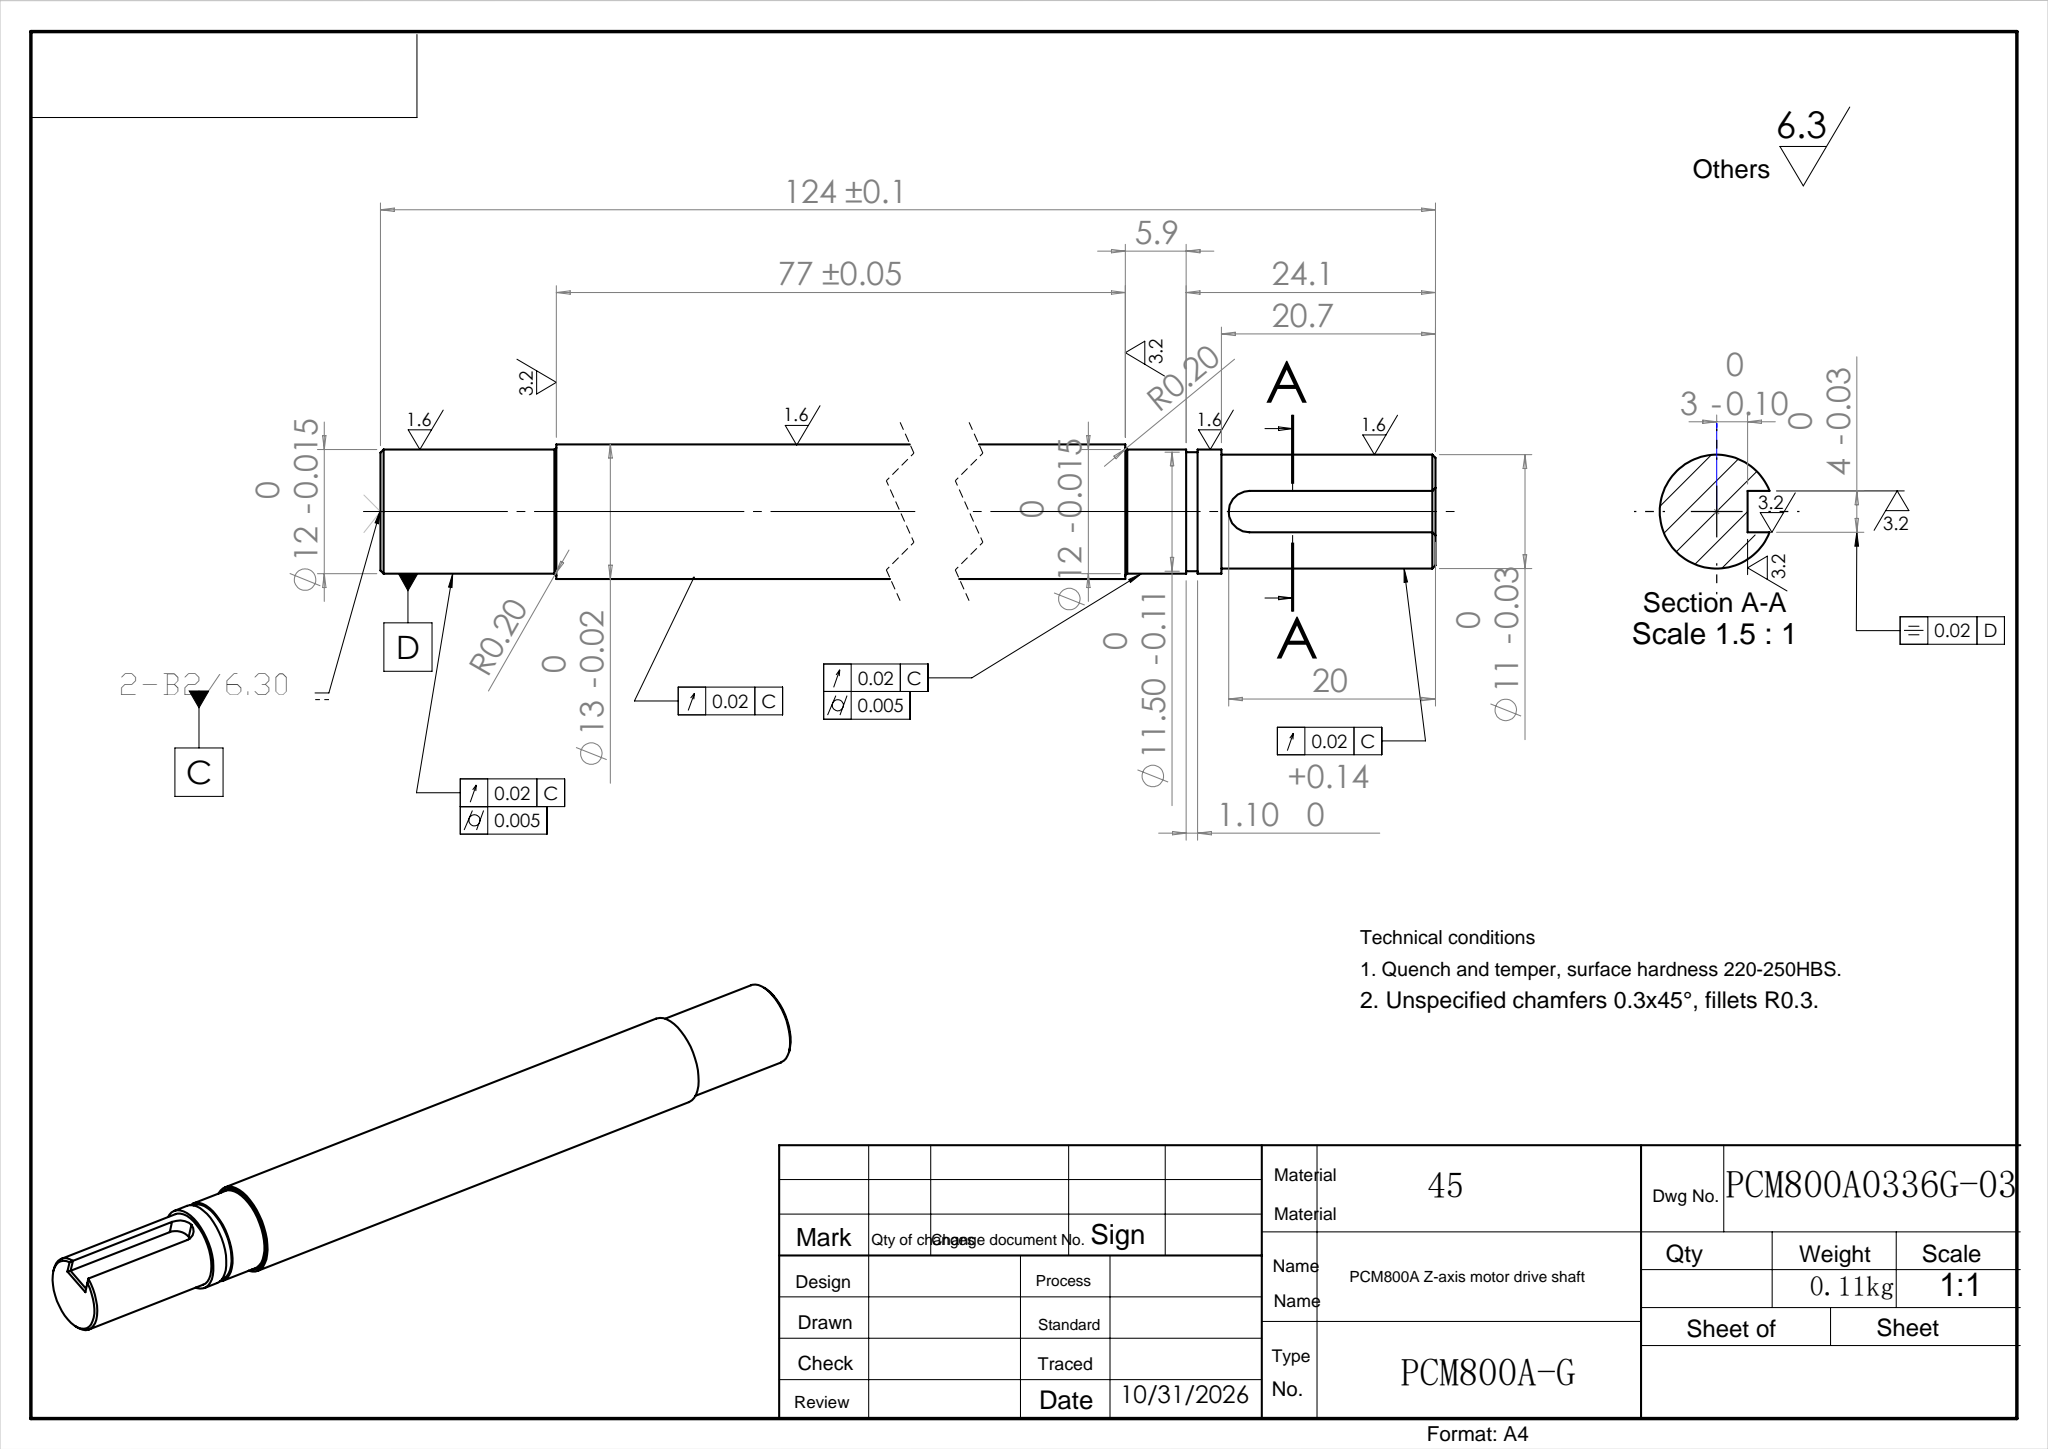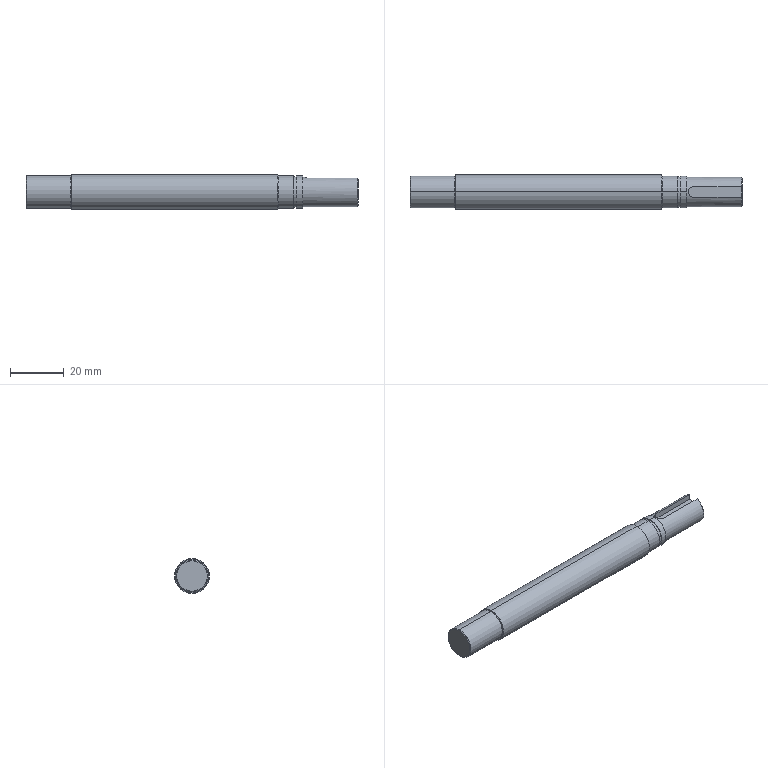Part | SolidWorks | features Boss 6, Fillet 3, Chamfer 1, Cut 1 | 1 solid | 34 faces | box 124 x 13 x 13 mm | volume 14963 mm3 | cylinder 14 | plane 13 | torus 4 | cone 3 | commonest cylinder face diameters 12 x6 4 x2 11 x2 11.5 x2 13 x2
STEP:
#1=CARTESIAN_POINT('',(77.2,0.,6.));
#2=VERTEX_POINT('',#1);
#3=CARTESIAN_POINT('',(77.2,0.,-6.));
#4=VERTEX_POINT('',#3);
#5=CARTESIAN_POINT('',(77.2,0.,0.));
#6=DIRECTION('',(1.,0.,0.));
#7=DIRECTION('',(0.,0.,-1.));
#8=AXIS2_PLACEMENT_3D('',#5,#6,#7);
#9=CIRCLE('',#8,6.);
#10=EDGE_CURVE('',#2,#4,#9,.T.);
#11=ORIENTED_EDGE('',*,*,#10,.F.);
#12=CARTESIAN_POINT('',(77.,0.,6.2));
#13=VERTEX_POINT('',#12);
#14=CARTESIAN_POINT('',(77.2,0.,6.2));
#15=DIRECTION('',(0.,1.,0.));
#16=DIRECTION('',(0.,0.,1.));
#17=AXIS2_PLACEMENT_3D('',#14,#15,#16);
#18=CIRCLE('',#17,0.2);
#19=EDGE_CURVE('',#2,#13,#18,.T.);
#20=ORIENTED_EDGE('',*,*,#19,.T.);
#21=CARTESIAN_POINT('',(77.,0.,-6.2));
#22=VERTEX_POINT('',#21);
#23=CARTESIAN_POINT('',(77.,0.,0.));
#24=DIRECTION('',(-1.,0.,0.));
#25=DIRECTION('',(0.,0.,-1.));
#26=AXIS2_PLACEMENT_3D('',#23,#24,#25);
#27=CIRCLE('',#26,6.2);
#28=EDGE_CURVE('',#22,#13,#27,.T.);
#29=ORIENTED_EDGE('',*,*,#28,.F.);
#30=CARTESIAN_POINT('',(77.2,0.,-6.2));
#31=DIRECTION('',(0.,-1.,0.));
#32=DIRECTION('',(0.,0.,-1.));
#33=AXIS2_PLACEMENT_3D('',#30,#31,#32);
#34=CIRCLE('',#33,0.2);
#35=EDGE_CURVE('',#4,#22,#34,.T.);
#36=ORIENTED_EDGE('',*,*,#35,.F.);
#37=EDGE_LOOP('',(#11,#20,#29,#36));
#38=FACE_OUTER_BOUND('',#37,.T.);
#39=CARTESIAN_POINT('',(77.2,0.,0.));
#40=DIRECTION('',(1.,0.,0.));
#41=DIRECTION('',(0.,0.,-1.));
#42=AXIS2_PLACEMENT_3D('',#39,#40,#41);
#43=TOROIDAL_SURFACE('',#42,6.2,0.2);
#44=ADVANCED_FACE('',(#38),#43,.F.);
#45=CARTESIAN_POINT('',(0.,0.,6.2));
#46=VERTEX_POINT('',#45);
#47=CARTESIAN_POINT('',(0.,0.,-6.2));
#48=VERTEX_POINT('',#47);
#49=CARTESIAN_POINT('',(0.,0.,0.));
#50=DIRECTION('',(1.,0.,0.));
#51=DIRECTION('',(0.,0.,-1.));
#52=AXIS2_PLACEMENT_3D('',#49,#50,#51);
#53=CIRCLE('',#52,6.2);
#54=EDGE_CURVE('',#46,#48,#53,.T.);
#55=ORIENTED_EDGE('',*,*,#54,.F.);
#56=CARTESIAN_POINT('',(-0.2,0.,6.));
#57=VERTEX_POINT('',#56);
#58=CARTESIAN_POINT('',(-0.2,0.,6.2));
#59=DIRECTION('',(0.,1.,0.));
#60=DIRECTION('',(0.,0.,1.));
#61=AXIS2_PLACEMENT_3D('',#58,#59,#60);
#62=CIRCLE('',#61,0.2);
#63=EDGE_CURVE('',#46,#57,#62,.T.);
#64=ORIENTED_EDGE('',*,*,#63,.T.);
#65=CARTESIAN_POINT('',(-0.2,0.,-6.));
#66=VERTEX_POINT('',#65);
#67=CARTESIAN_POINT('',(-0.2,0.,0.));
#68=DIRECTION('',(-1.,0.,0.));
#69=DIRECTION('',(0.,0.,-1.));
#70=AXIS2_PLACEMENT_3D('',#67,#68,#69);
#71=CIRCLE('',#70,6.);
#72=EDGE_CURVE('',#66,#57,#71,.T.);
#73=ORIENTED_EDGE('',*,*,#72,.F.);
#74=CARTESIAN_POINT('',(-0.2,0.,-6.2));
#75=DIRECTION('',(0.,-1.,0.));
#76=DIRECTION('',(0.,0.,-1.));
#77=AXIS2_PLACEMENT_3D('',#74,#75,#76);
#78=CIRCLE('',#77,0.2);
#79=EDGE_CURVE('',#48,#66,#78,.T.);
#80=ORIENTED_EDGE('',*,*,#79,.F.);
#81=EDGE_LOOP('',(#55,#64,#73,#80));
#82=FACE_OUTER_BOUND('',#81,.T.);
#83=CARTESIAN_POINT('',(-0.2,0.,0.));
#84=DIRECTION('',(1.,0.,0.));
#85=DIRECTION('',(0.,0.,-1.));
#86=AXIS2_PLACEMENT_3D('',#83,#84,#85);
#87=TOROIDAL_SURFACE('',#86,6.2,0.2);
#88=ADVANCED_FACE('',(#82),#87,.F.);
#89=CARTESIAN_POINT('',(-17.,0.,5.7));
#90=VERTEX_POINT('',#89);
#91=CARTESIAN_POINT('',(-17.,0.,-5.7));
#92=VERTEX_POINT('',#91);
#93=CARTESIAN_POINT('',(-17.,0.,0.));
#94=DIRECTION('',(-1.,0.,0.));
#95=DIRECTION('',(0.,0.,1.));
#96=AXIS2_PLACEMENT_3D('',#93,#94,#95);
#97=CIRCLE('',#96,5.7);
#98=EDGE_CURVE('',#90,#92,#97,.T.);
#99=ORIENTED_EDGE('',*,*,#98,.F.);
#100=CARTESIAN_POINT('',(-16.7,0.,6.));
#101=VERTEX_POINT('',#100);
#102=CARTESIAN_POINT('',(-17.,0.,5.7));
#103=DIRECTION('',(0.7071,0.,0.7071));
#104=VECTOR('',#103,1000.);
#105=LINE('',#102,#104);
#106=EDGE_CURVE('',#90,#101,#105,.T.);
#107=ORIENTED_EDGE('',*,*,#106,.T.);
#108=CARTESIAN_POINT('',(-16.7,0.,-6.));
#109=VERTEX_POINT('',#108);
#110=CARTESIAN_POINT('',(-16.7,0.,0.));
#111=DIRECTION('',(1.,0.,0.));
#112=DIRECTION('',(0.,0.,1.));
#113=AXIS2_PLACEMENT_3D('',#110,#111,#112);
#114=CIRCLE('',#113,6.);
#115=EDGE_CURVE('',#109,#101,#114,.T.);
#116=ORIENTED_EDGE('',*,*,#115,.F.);
#117=CARTESIAN_POINT('',(-17.,0.,-5.7));
#118=DIRECTION('',(0.7071,0.,-0.7071));
#119=VECTOR('',#118,1000.);
#120=LINE('',#117,#119);
#121=EDGE_CURVE('',#92,#109,#120,.T.);
#122=ORIENTED_EDGE('',*,*,#121,.F.);
#123=EDGE_LOOP('',(#99,#107,#116,#122));
#124=FACE_OUTER_BOUND('',#123,.T.);
#125=CARTESIAN_POINT('',(-17.,0.,0.));
#126=DIRECTION('',(1.,0.,0.));
#127=DIRECTION('',(0.,0.,-1.));
#128=AXIS2_PLACEMENT_3D('',#125,#126,#127);
#129=CONICAL_SURFACE('',#128,5.7,0.7854);
#130=ADVANCED_FACE('',(#124),#129,.T.);
#131=ORIENTED_EDGE('',*,*,#115,.T.);
#132=CARTESIAN_POINT('',(-17.,0.,6.));
#133=DIRECTION('',(1.,0.,0.));
#134=VECTOR('',#133,1000.);
#135=LINE('',#132,#134);
#136=EDGE_CURVE('',#101,#57,#135,.T.);
#137=ORIENTED_EDGE('',*,*,#136,.T.);
#138=CARTESIAN_POINT('',(-0.2,0.,0.));
#139=DIRECTION('',(-1.,0.,0.));
#140=DIRECTION('',(0.,0.,-1.));
#141=AXIS2_PLACEMENT_3D('',#138,#139,#140);
#142=CIRCLE('',#141,6.);
#143=EDGE_CURVE('',#57,#66,#142,.T.);
#144=ORIENTED_EDGE('',*,*,#143,.T.);
#145=CARTESIAN_POINT('',(-17.,0.,-6.));
#146=DIRECTION('',(1.,0.,0.));
#147=VECTOR('',#146,1000.);
#148=LINE('',#145,#147);
#149=EDGE_CURVE('',#109,#66,#148,.T.);
#150=ORIENTED_EDGE('',*,*,#149,.F.);
#151=EDGE_LOOP('',(#131,#137,#144,#150));
#152=FACE_OUTER_BOUND('',#151,.T.);
#153=CARTESIAN_POINT('',(-17.,0.,0.));
#154=DIRECTION('',(1.,0.,0.));
#155=DIRECTION('',(0.,0.,-1.));
#156=AXIS2_PLACEMENT_3D('',#153,#154,#155);
#157=CYLINDRICAL_SURFACE('',#156,6.);
#158=ADVANCED_FACE('',(#152),#157,.T.);
#159=CARTESIAN_POINT('',(106.7,2.,5.123));
#160=VERTEX_POINT('',#159);
#161=CARTESIAN_POINT('',(106.7,0.,-5.5));
#162=VERTEX_POINT('',#161);
#163=CARTESIAN_POINT('',(106.7,0.,0.));
#164=DIRECTION('',(-1.,0.,0.));
#165=DIRECTION('',(0.,0.,-1.));
#166=AXIS2_PLACEMENT_3D('',#163,#164,#165);
#167=CIRCLE('',#166,5.5);
#168=EDGE_CURVE('',#160,#162,#167,.T.);
#169=ORIENTED_EDGE('',*,*,#168,.T.);
#170=CARTESIAN_POINT('',(86.3,0.,-5.5));
#171=VERTEX_POINT('',#170);
#172=CARTESIAN_POINT('',(107.,0.,-5.5));
#173=DIRECTION('',(-1.,0.,0.));
#174=VECTOR('',#173,1000.);
#175=LINE('',#172,#174);
#176=EDGE_CURVE('',#162,#171,#175,.T.);
#177=ORIENTED_EDGE('',*,*,#176,.T.);
#178=CARTESIAN_POINT('',(86.3,0.,5.5));
#179=VERTEX_POINT('',#178);
#180=CARTESIAN_POINT('',(86.3,0.,0.));
#181=DIRECTION('',(1.,0.,0.));
#182=DIRECTION('',(0.,0.,-1.));
#183=AXIS2_PLACEMENT_3D('',#180,#181,#182);
#184=CIRCLE('',#183,5.5);
#185=EDGE_CURVE('',#171,#179,#184,.T.);
#186=ORIENTED_EDGE('',*,*,#185,.T.);
#187=CARTESIAN_POINT('',(87.,0.,5.5));
#188=VERTEX_POINT('',#187);
#189=CARTESIAN_POINT('',(107.,0.,5.5));
#190=DIRECTION('',(-1.,0.,0.));
#191=VECTOR('',#190,1000.);
#192=LINE('',#189,#191);
#193=EDGE_CURVE('',#188,#179,#192,.T.);
#194=ORIENTED_EDGE('',*,*,#193,.F.);
#195=CARTESIAN_POINT('',(89.,2.,5.123));
#196=VERTEX_POINT('',#195);
#197=CARTESIAN_POINT('',(87.,0.,5.5));
#198=CARTESIAN_POINT('',(87.,0.1333,5.5));
#199=CARTESIAN_POINT('',(87.013,0.2641,5.495));
#200=CARTESIAN_POINT('',(87.065,0.5212,5.477));
#201=CARTESIAN_POINT('',(87.104,0.6488,5.463));
#202=CARTESIAN_POINT('',(87.204,0.8905,5.429));
#203=CARTESIAN_POINT('',(87.266,1.005,5.409));
#204=CARTESIAN_POINT('',(87.411,1.221,5.364));
#205=CARTESIAN_POINT('',(87.494,1.323,5.339));
#206=CARTESIAN_POINT('',(87.769,1.597,5.266));
#207=CARTESIAN_POINT('',(87.989,1.745,5.217));
#208=CARTESIAN_POINT('',(88.349,1.896,5.163));
#209=CARTESIAN_POINT('',(88.476,1.935,5.149));
#210=CARTESIAN_POINT('',(88.735,1.987,5.129));
#211=CARTESIAN_POINT('',(88.867,2.,5.123));
#212=CARTESIAN_POINT('',(89.,2.,5.123));
#213=B_SPLINE_CURVE_WITH_KNOTS('',3,(#197,#198,#199,#200,#201,#202,#203,#204,#205,#206,#207,#208,#209,#210,#211,#212),.UNSPECIFIED.,.F.,.F.,(4,2,2,2,2,2,2,4),(0.,0.000394,0.0007879,0.001182,0.001576,0.002364,0.002758,0.003152),.UNSPECIFIED.);
#214=EDGE_CURVE('',#188,#196,#213,.T.);
#215=ORIENTED_EDGE('',*,*,#214,.T.);
#216=CARTESIAN_POINT('',(87.,2.,5.123));
#217=DIRECTION('',(1.,0.,0.));
#218=VECTOR('',#217,1000.);
#219=LINE('',#216,#218);
#220=EDGE_CURVE('',#196,#160,#219,.T.);
#221=ORIENTED_EDGE('',*,*,#220,.T.);
#222=EDGE_LOOP('',(#169,#177,#186,#194,#215,#221));
#223=FACE_OUTER_BOUND('',#222,.T.);
#224=CARTESIAN_POINT('',(107.,0.,0.));
#225=DIRECTION('',(-1.,0.,0.));
#226=DIRECTION('',(0.,0.,1.));
#227=AXIS2_PLACEMENT_3D('',#224,#225,#226);
#228=CYLINDRICAL_SURFACE('',#227,5.5);
#229=ADVANCED_FACE('',(#223),#228,.T.);
#230=CARTESIAN_POINT('',(86.3,0.,-6.));
#231=VERTEX_POINT('',#230);
#232=CARTESIAN_POINT('',(86.3,0.,6.));
#233=VERTEX_POINT('',#232);
#234=CARTESIAN_POINT('',(86.3,0.,0.));
#235=DIRECTION('',(1.,0.,0.));
#236=DIRECTION('',(0.,0.,-1.));
#237=AXIS2_PLACEMENT_3D('',#234,#235,#236);
#238=CIRCLE('',#237,6.);
#239=EDGE_CURVE('',#231,#233,#238,.T.);
#240=ORIENTED_EDGE('',*,*,#239,.F.);
#241=CARTESIAN_POINT('',(84.,0.,-6.));
#242=VERTEX_POINT('',#241);
#243=CARTESIAN_POINT('',(86.3,0.,-6.));
#244=DIRECTION('',(-1.,0.,0.));
#245=VECTOR('',#244,1000.);
#246=LINE('',#243,#245);
#247=EDGE_CURVE('',#231,#242,#246,.T.);
#248=ORIENTED_EDGE('',*,*,#247,.T.);
#249=CARTESIAN_POINT('',(84.,0.,6.));
#250=VERTEX_POINT('',#249);
#251=CARTESIAN_POINT('',(84.,0.,0.));
#252=DIRECTION('',(1.,0.,0.));
#253=DIRECTION('',(0.,0.,-1.));
#254=AXIS2_PLACEMENT_3D('',#251,#252,#253);
#255=CIRCLE('',#254,6.);
#256=EDGE_CURVE('',#242,#250,#255,.T.);
#257=ORIENTED_EDGE('',*,*,#256,.T.);
#258=CARTESIAN_POINT('',(86.3,0.,6.));
#259=DIRECTION('',(-1.,0.,0.));
#260=VECTOR('',#259,1000.);
#261=LINE('',#258,#260);
#262=EDGE_CURVE('',#233,#250,#261,.T.);
#263=ORIENTED_EDGE('',*,*,#262,.F.);
#264=EDGE_LOOP('',(#240,#248,#257,#263));
#265=FACE_OUTER_BOUND('',#264,.T.);
#266=CARTESIAN_POINT('',(86.3,0.,0.));
#267=DIRECTION('',(-1.,0.,0.));
#268=DIRECTION('',(0.,0.,1.));
#269=AXIS2_PLACEMENT_3D('',#266,#267,#268);
#270=CYLINDRICAL_SURFACE('',#269,6.);
#271=ADVANCED_FACE('',(#265),#270,.T.);
#272=CARTESIAN_POINT('',(84.,0.,-5.75));
#273=VERTEX_POINT('',#272);
#274=CARTESIAN_POINT('',(84.,0.,5.75));
#275=VERTEX_POINT('',#274);
#276=CARTESIAN_POINT('',(84.,0.,0.));
#277=DIRECTION('',(1.,0.,0.));
#278=DIRECTION('',(0.,0.,-1.));
#279=AXIS2_PLACEMENT_3D('',#276,#277,#278);
#280=CIRCLE('',#279,5.75);
#281=EDGE_CURVE('',#273,#275,#280,.T.);
#282=ORIENTED_EDGE('',*,*,#281,.F.);
#283=CARTESIAN_POINT('',(82.9,0.,-5.75));
#284=VERTEX_POINT('',#283);
#285=CARTESIAN_POINT('',(84.,0.,-5.75));
#286=DIRECTION('',(-1.,0.,0.));
#287=VECTOR('',#286,1000.);
#288=LINE('',#285,#287);
#289=EDGE_CURVE('',#273,#284,#288,.T.);
#290=ORIENTED_EDGE('',*,*,#289,.T.);
#291=CARTESIAN_POINT('',(82.9,0.,5.75));
#292=VERTEX_POINT('',#291);
#293=CARTESIAN_POINT('',(82.9,0.,0.));
#294=DIRECTION('',(1.,0.,0.));
#295=DIRECTION('',(0.,0.,-1.));
#296=AXIS2_PLACEMENT_3D('',#293,#294,#295);
#297=CIRCLE('',#296,5.75);
#298=EDGE_CURVE('',#284,#292,#297,.T.);
#299=ORIENTED_EDGE('',*,*,#298,.T.);
#300=CARTESIAN_POINT('',(84.,0.,5.75));
#301=DIRECTION('',(-1.,0.,0.));
#302=VECTOR('',#301,1000.);
#303=LINE('',#300,#302);
#304=EDGE_CURVE('',#275,#292,#303,.T.);
#305=ORIENTED_EDGE('',*,*,#304,.F.);
#306=EDGE_LOOP('',(#282,#290,#299,#305));
#307=FACE_OUTER_BOUND('',#306,.T.);
#308=CARTESIAN_POINT('',(84.,0.,0.));
#309=DIRECTION('',(-1.,0.,0.));
#310=DIRECTION('',(0.,0.,1.));
#311=AXIS2_PLACEMENT_3D('',#308,#309,#310);
#312=CYLINDRICAL_SURFACE('',#311,5.75);
#313=ADVANCED_FACE('',(#307),#312,.T.);
#314=CARTESIAN_POINT('',(82.9,0.,-6.));
#315=VERTEX_POINT('',#314);
#316=CARTESIAN_POINT('',(82.9,0.,6.));
#317=VERTEX_POINT('',#316);
#318=CARTESIAN_POINT('',(82.9,0.,0.));
#319=DIRECTION('',(1.,0.,0.));
#320=DIRECTION('',(0.,0.,-1.));
#321=AXIS2_PLACEMENT_3D('',#318,#319,#320);
#322=CIRCLE('',#321,6.);
#323=EDGE_CURVE('',#315,#317,#322,.T.);
#324=ORIENTED_EDGE('',*,*,#323,.F.);
#325=CARTESIAN_POINT('',(82.9,0.,-6.));
#326=DIRECTION('',(-1.,0.,0.));
#327=VECTOR('',#326,1000.);
#328=LINE('',#325,#327);
#329=EDGE_CURVE('',#315,#4,#328,.T.);
#330=ORIENTED_EDGE('',*,*,#329,.T.);
#331=CARTESIAN_POINT('',(77.2,0.,0.));
#332=DIRECTION('',(1.,0.,0.));
#333=DIRECTION('',(0.,0.,-1.));
#334=AXIS2_PLACEMENT_3D('',#331,#332,#333);
#335=CIRCLE('',#334,6.);
#336=EDGE_CURVE('',#4,#2,#335,.T.);
#337=ORIENTED_EDGE('',*,*,#336,.T.);
#338=CARTESIAN_POINT('',(82.9,0.,6.));
#339=DIRECTION('',(-1.,0.,0.));
#340=VECTOR('',#339,1000.);
#341=LINE('',#338,#340);
#342=EDGE_CURVE('',#317,#2,#341,.T.);
#343=ORIENTED_EDGE('',*,*,#342,.F.);
#344=EDGE_LOOP('',(#324,#330,#337,#343));
#345=FACE_OUTER_BOUND('',#344,.T.);
#346=CARTESIAN_POINT('',(82.9,0.,0.));
#347=DIRECTION('',(-1.,0.,0.));
#348=DIRECTION('',(0.,0.,1.));
#349=AXIS2_PLACEMENT_3D('',#346,#347,#348);
#350=CYLINDRICAL_SURFACE('',#349,6.);
#351=ADVANCED_FACE('',(#345),#350,.T.);
#352=CARTESIAN_POINT('',(77.,0.,-6.5));
#353=VERTEX_POINT('',#352);
#354=CARTESIAN_POINT('',(77.,0.,6.5));
#355=VERTEX_POINT('',#354);
#356=CARTESIAN_POINT('',(77.,0.,0.));
#357=DIRECTION('',(1.,0.,0.));
#358=DIRECTION('',(0.,0.,-1.));
#359=AXIS2_PLACEMENT_3D('',#356,#357,#358);
#360=CIRCLE('',#359,6.5);
#361=EDGE_CURVE('',#353,#355,#360,.T.);
#362=ORIENTED_EDGE('',*,*,#361,.F.);
#363=CARTESIAN_POINT('',(0.,0.,-6.5));
#364=VERTEX_POINT('',#363);
#365=CARTESIAN_POINT('',(77.,0.,-6.5));
#366=DIRECTION('',(-1.,0.,0.));
#367=VECTOR('',#366,1000.);
#368=LINE('',#365,#367);
#369=EDGE_CURVE('',#353,#364,#368,.T.);
#370=ORIENTED_EDGE('',*,*,#369,.T.);
#371=CARTESIAN_POINT('',(0.,0.,6.5));
#372=VERTEX_POINT('',#371);
#373=CARTESIAN_POINT('',(0.,0.,0.));
#374=DIRECTION('',(1.,0.,0.));
#375=DIRECTION('',(0.,0.,-1.));
#376=AXIS2_PLACEMENT_3D('',#373,#374,#375);
#377=CIRCLE('',#376,6.5);
#378=EDGE_CURVE('',#364,#372,#377,.T.);
#379=ORIENTED_EDGE('',*,*,#378,.T.);
#380=CARTESIAN_POINT('',(77.,0.,6.5));
#381=DIRECTION('',(-1.,0.,0.));
#382=VECTOR('',#381,1000.);
#383=LINE('',#380,#382);
#384=EDGE_CURVE('',#355,#372,#383,.T.);
#385=ORIENTED_EDGE('',*,*,#384,.F.);
#386=EDGE_LOOP('',(#362,#370,#379,#385));
#387=FACE_OUTER_BOUND('',#386,.T.);
#388=CARTESIAN_POINT('',(77.,0.,0.));
#389=DIRECTION('',(-1.,0.,0.));
#390=DIRECTION('',(0.,0.,1.));
#391=AXIS2_PLACEMENT_3D('',#388,#389,#390);
#392=CYLINDRICAL_SURFACE('',#391,6.5);
#393=ADVANCED_FACE('',(#387),#392,.T.);
#394=CARTESIAN_POINT('',(0.,0.,0.));
#395=DIRECTION('',(1.,0.,0.));
#396=DIRECTION('',(0.,0.,-1.));
#397=AXIS2_PLACEMENT_3D('',#394,#395,#396);
#398=CIRCLE('',#397,6.2);
#399=EDGE_CURVE('',#48,#46,#398,.T.);
#400=ORIENTED_EDGE('',*,*,#399,.T.);
#401=ORIENTED_EDGE('',*,*,#54,.T.);
#402=EDGE_LOOP('',(#400,#401));
#403=FACE_BOUND('',#402,.T.);
#404=CARTESIAN_POINT('',(0.,0.,0.));
#405=DIRECTION('',(1.,0.,0.));
#406=DIRECTION('',(0.,0.,-1.));
#407=AXIS2_PLACEMENT_3D('',#404,#405,#406);
#408=CIRCLE('',#407,6.5);
#409=EDGE_CURVE('',#372,#364,#408,.T.);
#410=ORIENTED_EDGE('',*,*,#409,.F.);
#411=ORIENTED_EDGE('',*,*,#378,.F.);
#412=EDGE_LOOP('',(#410,#411));
#413=FACE_OUTER_BOUND('',#412,.T.);
#414=CARTESIAN_POINT('',(0.,0.,0.));
#415=DIRECTION('',(1.,0.,0.));
#416=DIRECTION('',(0.,0.,-1.));
#417=AXIS2_PLACEMENT_3D('',#414,#415,#416);
#418=PLANE('',#417);
#419=ADVANCED_FACE('',(#403,#413),#418,.F.);
#420=CARTESIAN_POINT('',(86.3,0.,0.));
#421=DIRECTION('',(1.,0.,0.));
#422=DIRECTION('',(0.,0.,-1.));
#423=AXIS2_PLACEMENT_3D('',#420,#421,#422);
#424=CIRCLE('',#423,6.);
#425=EDGE_CURVE('',#233,#231,#424,.T.);
#426=ORIENTED_EDGE('',*,*,#425,.T.);
#427=ORIENTED_EDGE('',*,*,#239,.T.);
#428=EDGE_LOOP('',(#426,#427));
#429=FACE_OUTER_BOUND('',#428,.T.);
#430=CARTESIAN_POINT('',(86.3,0.,0.));
#431=DIRECTION('',(1.,0.,0.));
#432=DIRECTION('',(0.,0.,-1.));
#433=AXIS2_PLACEMENT_3D('',#430,#431,#432);
#434=CIRCLE('',#433,5.5);
#435=EDGE_CURVE('',#179,#171,#434,.T.);
#436=ORIENTED_EDGE('',*,*,#435,.F.);
#437=ORIENTED_EDGE('',*,*,#185,.F.);
#438=EDGE_LOOP('',(#436,#437));
#439=FACE_BOUND('',#438,.T.);
#440=CARTESIAN_POINT('',(86.3,0.,0.));
#441=DIRECTION('',(1.,0.,0.));
#442=DIRECTION('',(0.,0.,-1.));
#443=AXIS2_PLACEMENT_3D('',#440,#441,#442);
#444=PLANE('',#443);
#445=ADVANCED_FACE('',(#429,#439),#444,.T.);
#446=CARTESIAN_POINT('',(82.9,0.,0.));
#447=DIRECTION('',(1.,0.,0.));
#448=DIRECTION('',(0.,0.,-1.));
#449=AXIS2_PLACEMENT_3D('',#446,#447,#448);
#450=CIRCLE('',#449,6.);
#451=EDGE_CURVE('',#317,#315,#450,.T.);
#452=ORIENTED_EDGE('',*,*,#451,.T.);
#453=ORIENTED_EDGE('',*,*,#323,.T.);
#454=EDGE_LOOP('',(#452,#453));
#455=FACE_OUTER_BOUND('',#454,.T.);
#456=CARTESIAN_POINT('',(82.9,0.,0.));
#457=DIRECTION('',(1.,0.,0.));
#458=DIRECTION('',(0.,0.,-1.));
#459=AXIS2_PLACEMENT_3D('',#456,#457,#458);
#460=CIRCLE('',#459,5.75);
#461=EDGE_CURVE('',#292,#284,#460,.T.);
#462=ORIENTED_EDGE('',*,*,#461,.F.);
#463=ORIENTED_EDGE('',*,*,#298,.F.);
#464=EDGE_LOOP('',(#462,#463));
#465=FACE_BOUND('',#464,.T.);
#466=CARTESIAN_POINT('',(82.9,0.,0.));
#467=DIRECTION('',(1.,0.,0.));
#468=DIRECTION('',(0.,0.,-1.));
#469=AXIS2_PLACEMENT_3D('',#466,#467,#468);
#470=PLANE('',#469);
#471=ADVANCED_FACE('',(#455,#465),#470,.T.);
#472=ORIENTED_EDGE('',*,*,#28,.T.);
#473=CARTESIAN_POINT('',(77.,0.,0.));
#474=DIRECTION('',(-1.,0.,0.));
#475=DIRECTION('',(0.,0.,-1.));
#476=AXIS2_PLACEMENT_3D('',#473,#474,#475);
#477=CIRCLE('',#476,6.2);
#478=EDGE_CURVE('',#13,#22,#477,.T.);
#479=ORIENTED_EDGE('',*,*,#478,.T.);
#480=EDGE_LOOP('',(#472,#479));
#481=FACE_BOUND('',#480,.T.);
#482=CARTESIAN_POINT('',(77.,0.,0.));
#483=DIRECTION('',(1.,0.,0.));
#484=DIRECTION('',(0.,0.,-1.));
#485=AXIS2_PLACEMENT_3D('',#482,#483,#484);
#486=CIRCLE('',#485,6.5);
#487=EDGE_CURVE('',#355,#353,#486,.T.);
#488=ORIENTED_EDGE('',*,*,#487,.T.);
#489=ORIENTED_EDGE('',*,*,#361,.T.);
#490=EDGE_LOOP('',(#488,#489));
#491=FACE_OUTER_BOUND('',#490,.T.);
#492=CARTESIAN_POINT('',(77.,0.,0.));
#493=DIRECTION('',(1.,0.,0.));
#494=DIRECTION('',(0.,0.,-1.));
#495=AXIS2_PLACEMENT_3D('',#492,#493,#494);
#496=PLANE('',#495);
#497=ADVANCED_FACE('',(#481,#491),#496,.T.);
#498=ORIENTED_EDGE('',*,*,#369,.F.);
#499=ORIENTED_EDGE('',*,*,#487,.F.);
#500=ORIENTED_EDGE('',*,*,#384,.T.);
#501=ORIENTED_EDGE('',*,*,#409,.T.);
#502=EDGE_LOOP('',(#498,#499,#500,#501));
#503=FACE_OUTER_BOUND('',#502,.T.);
#504=CARTESIAN_POINT('',(77.,0.,0.));
#505=DIRECTION('',(-1.,0.,0.));
#506=DIRECTION('',(0.,0.,1.));
#507=AXIS2_PLACEMENT_3D('',#504,#505,#506);
#508=CYLINDRICAL_SURFACE('',#507,6.5);
#509=ADVANCED_FACE('',(#503),#508,.T.);
#510=ORIENTED_EDGE('',*,*,#329,.F.);
#511=ORIENTED_EDGE('',*,*,#451,.F.);
#512=ORIENTED_EDGE('',*,*,#342,.T.);
#513=ORIENTED_EDGE('',*,*,#10,.T.);
#514=EDGE_LOOP('',(#510,#511,#512,#513));
#515=FACE_OUTER_BOUND('',#514,.T.);
#516=CARTESIAN_POINT('',(82.9,0.,0.));
#517=DIRECTION('',(-1.,0.,0.));
#518=DIRECTION('',(0.,0.,1.));
#519=AXIS2_PLACEMENT_3D('',#516,#517,#518);
#520=CYLINDRICAL_SURFACE('',#519,6.);
#521=ADVANCED_FACE('',(#515),#520,.T.);
#522=ORIENTED_EDGE('',*,*,#289,.F.);
#523=CARTESIAN_POINT('',(84.,0.,0.));
#524=DIRECTION('',(1.,0.,0.));
#525=DIRECTION('',(0.,0.,-1.));
#526=AXIS2_PLACEMENT_3D('',#523,#524,#525);
#527=CIRCLE('',#526,5.75);
#528=EDGE_CURVE('',#275,#273,#527,.T.);
#529=ORIENTED_EDGE('',*,*,#528,.F.);
#530=ORIENTED_EDGE('',*,*,#304,.T.);
#531=ORIENTED_EDGE('',*,*,#461,.T.);
#532=EDGE_LOOP('',(#522,#529,#530,#531));
#533=FACE_OUTER_BOUND('',#532,.T.);
#534=CARTESIAN_POINT('',(84.,0.,0.));
#535=DIRECTION('',(-1.,0.,0.));
#536=DIRECTION('',(0.,0.,1.));
#537=AXIS2_PLACEMENT_3D('',#534,#535,#536);
#538=CYLINDRICAL_SURFACE('',#537,5.75);
#539=ADVANCED_FACE('',(#533),#538,.T.);
#540=CARTESIAN_POINT('',(84.,0.,0.));
#541=DIRECTION('',(1.,0.,0.));
#542=DIRECTION('',(0.,0.,-1.));
#543=AXIS2_PLACEMENT_3D('',#540,#541,#542);
#544=CIRCLE('',#543,6.);
#545=EDGE_CURVE('',#250,#242,#544,.T.);
#546=ORIENTED_EDGE('',*,*,#545,.F.);
#547=ORIENTED_EDGE('',*,*,#256,.F.);
#548=EDGE_LOOP('',(#546,#547));
#549=FACE_OUTER_BOUND('',#548,.T.);
#550=ORIENTED_EDGE('',*,*,#528,.T.);
#551=ORIENTED_EDGE('',*,*,#281,.T.);
#552=EDGE_LOOP('',(#550,#551));
#553=FACE_BOUND('',#552,.T.);
#554=CARTESIAN_POINT('',(84.,0.,0.));
#555=DIRECTION('',(1.,0.,0.));
#556=DIRECTION('',(0.,0.,-1.));
#557=AXIS2_PLACEMENT_3D('',#554,#555,#556);
#558=PLANE('',#557);
#559=ADVANCED_FACE('',(#549,#553),#558,.F.);
#560=ORIENTED_EDGE('',*,*,#247,.F.);
#561=ORIENTED_EDGE('',*,*,#425,.F.);
#562=ORIENTED_EDGE('',*,*,#262,.T.);
#563=ORIENTED_EDGE('',*,*,#545,.T.);
#564=EDGE_LOOP('',(#560,#561,#562,#563));
#565=FACE_OUTER_BOUND('',#564,.T.);
#566=CARTESIAN_POINT('',(86.3,0.,0.));
#567=DIRECTION('',(-1.,0.,0.));
#568=DIRECTION('',(0.,0.,1.));
#569=AXIS2_PLACEMENT_3D('',#566,#567,#568);
#570=CYLINDRICAL_SURFACE('',#569,6.);
#571=ADVANCED_FACE('',(#565),#570,.T.);
#572=ORIENTED_EDGE('',*,*,#176,.F.);
#573=CARTESIAN_POINT('',(106.7,-2.,5.123));
#574=VERTEX_POINT('',#573);
#575=CARTESIAN_POINT('',(106.7,0.,0.));
#576=DIRECTION('',(-1.,0.,0.));
#577=DIRECTION('',(0.,0.,-1.));
#578=AXIS2_PLACEMENT_3D('',#575,#576,#577);
#579=CIRCLE('',#578,5.5);
#580=EDGE_CURVE('',#162,#574,#579,.T.);
#581=ORIENTED_EDGE('',*,*,#580,.T.);
#582=CARTESIAN_POINT('',(89.,-2.,5.123));
#583=VERTEX_POINT('',#582);
#584=CARTESIAN_POINT('',(87.,-2.,5.123));
#585=DIRECTION('',(1.,0.,0.));
#586=VECTOR('',#585,1000.);
#587=LINE('',#584,#586);
#588=EDGE_CURVE('',#583,#574,#587,.T.);
#589=ORIENTED_EDGE('',*,*,#588,.F.);
#590=CARTESIAN_POINT('',(89.,-2.,5.123));
#591=CARTESIAN_POINT('',(88.867,-2.,5.123));
#592=CARTESIAN_POINT('',(88.736,-1.987,5.129));
#593=CARTESIAN_POINT('',(88.479,-1.935,5.148));
#594=CARTESIAN_POINT('',(88.351,-1.896,5.163));
#595=CARTESIAN_POINT('',(88.11,-1.796,5.199));
#596=CARTESIAN_POINT('',(87.996,-1.734,5.22));
#597=CARTESIAN_POINT('',(87.779,-1.589,5.266));
#598=CARTESIAN_POINT('',(87.678,-1.506,5.291));
#599=CARTESIAN_POINT('',(87.404,-1.232,5.364));
#600=CARTESIAN_POINT('',(87.255,-1.011,5.412));
#601=CARTESIAN_POINT('',(87.104,-0.6509,5.463));
#602=CARTESIAN_POINT('',(87.065,-0.524,5.477));
#603=CARTESIAN_POINT('',(87.013,-0.2647,5.495));
#604=CARTESIAN_POINT('',(87.,-0.1333,5.5));
#605=CARTESIAN_POINT('',(87.,0.,5.5));
#606=B_SPLINE_CURVE_WITH_KNOTS('',3,(#590,#591,#592,#593,#594,#595,#596,#597,#598,#599,#600,#601,#602,#603,#604,#605),.UNSPECIFIED.,.F.,.F.,(4,2,2,2,2,2,2,4),(0.,0.000394,0.0007879,0.001182,0.001576,0.002364,0.002758,0.003152),.UNSPECIFIED.);
#607=EDGE_CURVE('',#583,#188,#606,.T.);
#608=ORIENTED_EDGE('',*,*,#607,.T.);
#609=ORIENTED_EDGE('',*,*,#193,.T.);
#610=ORIENTED_EDGE('',*,*,#435,.T.);
#611=EDGE_LOOP('',(#572,#581,#589,#608,#609,#610));
#612=FACE_OUTER_BOUND('',#611,.T.);
#613=CARTESIAN_POINT('',(107.,0.,0.));
#614=DIRECTION('',(-1.,0.,0.));
#615=DIRECTION('',(0.,0.,1.));
#616=AXIS2_PLACEMENT_3D('',#613,#614,#615);
#617=CYLINDRICAL_SURFACE('',#616,5.5);
#618=ADVANCED_FACE('',(#612),#617,.T.);
#619=CARTESIAN_POINT('',(107.,-2.3,2.7));
#620=VERTEX_POINT('',#619);
#621=CARTESIAN_POINT('',(107.,-2.3,4.664));
#622=VERTEX_POINT('',#621);
#623=CARTESIAN_POINT('',(107.,-2.3,5.123));
#624=DIRECTION('',(0.,0.,1.));
#625=VECTOR('',#624,1000.);
#626=LINE('',#623,#625);
#627=EDGE_CURVE('',#620,#622,#626,.T.);
#628=ORIENTED_EDGE('',*,*,#627,.T.);
#629=CARTESIAN_POINT('',(107.,2.3,4.664));
#630=VERTEX_POINT('',#629);
#631=CARTESIAN_POINT('',(107.,0.,0.));
#632=DIRECTION('',(1.,0.,0.));
#633=DIRECTION('',(0.,0.,-1.));
#634=AXIS2_PLACEMENT_3D('',#631,#632,#633);
#635=CIRCLE('',#634,5.2);
#636=EDGE_CURVE('',#622,#630,#635,.T.);
#637=ORIENTED_EDGE('',*,*,#636,.T.);
#638=CARTESIAN_POINT('',(107.,2.3,2.7));
#639=VERTEX_POINT('',#638);
#640=CARTESIAN_POINT('',(107.,2.3,3.));
#641=DIRECTION('',(0.,0.,-1.));
#642=VECTOR('',#641,1000.);
#643=LINE('',#640,#642);
#644=EDGE_CURVE('',#630,#639,#643,.T.);
#645=ORIENTED_EDGE('',*,*,#644,.T.);
#646=CARTESIAN_POINT('',(107.,-2.,2.7));
#647=DIRECTION('',(0.,-1.,0.));
#648=VECTOR('',#647,1000.);
#649=LINE('',#646,#648);
#650=EDGE_CURVE('',#639,#620,#649,.T.);
#651=ORIENTED_EDGE('',*,*,#650,.T.);
#652=EDGE_LOOP('',(#628,#637,#645,#651));
#653=FACE_OUTER_BOUND('',#652,.T.);
#654=CARTESIAN_POINT('',(107.,0.,0.));
#655=DIRECTION('',(1.,0.,0.));
#656=DIRECTION('',(0.,0.,-1.));
#657=AXIS2_PLACEMENT_3D('',#654,#655,#656);
#658=PLANE('',#657);
#659=ADVANCED_FACE('',(#653),#658,.T.);
#660=CARTESIAN_POINT('',(89.,2.,3.));
#661=VERTEX_POINT('',#660);
#662=CARTESIAN_POINT('',(106.7,2.,3.));
#663=VERTEX_POINT('',#662);
#664=CARTESIAN_POINT('',(87.,2.,3.));
#665=DIRECTION('',(1.,0.,0.));
#666=VECTOR('',#665,1000.);
#667=LINE('',#664,#666);
#668=EDGE_CURVE('',#661,#663,#667,.T.);
#669=ORIENTED_EDGE('',*,*,#668,.T.);
#670=CARTESIAN_POINT('',(106.7,2.,5.123));
#671=DIRECTION('',(0.,0.,1.));
#672=VECTOR('',#671,1000.);
#673=LINE('',#670,#672);
#674=EDGE_CURVE('',#663,#160,#673,.T.);
#675=ORIENTED_EDGE('',*,*,#674,.T.);
#676=ORIENTED_EDGE('',*,*,#220,.F.);
#677=CARTESIAN_POINT('',(89.,2.,3.));
#678=DIRECTION('',(0.,0.,-1.));
#679=VECTOR('',#678,1000.);
#680=LINE('',#677,#679);
#681=EDGE_CURVE('',#196,#661,#680,.T.);
#682=ORIENTED_EDGE('',*,*,#681,.T.);
#683=EDGE_LOOP('',(#669,#675,#676,#682));
#684=FACE_OUTER_BOUND('',#683,.T.);
#685=CARTESIAN_POINT('',(87.,2.,3.));
#686=DIRECTION('',(0.,1.,0.));
#687=DIRECTION('',(-1.,0.,0.));
#688=AXIS2_PLACEMENT_3D('',#685,#686,#687);
#689=PLANE('',#688);
#690=ADVANCED_FACE('',(#684),#689,.F.);
#691=CARTESIAN_POINT('',(89.,-2.,3.));
#692=VERTEX_POINT('',#691);
#693=CARTESIAN_POINT('',(106.7,-2.,3.));
#694=VERTEX_POINT('',#693);
#695=CARTESIAN_POINT('',(87.,-2.,3.));
#696=DIRECTION('',(1.,0.,0.));
#697=VECTOR('',#696,1000.);
#698=LINE('',#695,#697);
#699=EDGE_CURVE('',#692,#694,#698,.T.);
#700=ORIENTED_EDGE('',*,*,#699,.T.);
#701=CARTESIAN_POINT('',(106.7,2.,3.));
#702=DIRECTION('',(0.,1.,0.));
#703=VECTOR('',#702,1000.);
#704=LINE('',#701,#703);
#705=EDGE_CURVE('',#694,#663,#704,.T.);
#706=ORIENTED_EDGE('',*,*,#705,.T.);
#707=ORIENTED_EDGE('',*,*,#668,.F.);
#708=CARTESIAN_POINT('',(87.,0.,3.));
#709=VERTEX_POINT('',#708);
#710=CARTESIAN_POINT('',(89.,0.,3.));
#711=DIRECTION('',(0.,0.,1.));
#712=DIRECTION('',(-1.,0.,0.));
#713=AXIS2_PLACEMENT_3D('',#710,#711,#712);
#714=CIRCLE('',#713,2.);
#715=EDGE_CURVE('',#661,#709,#714,.T.);
#716=ORIENTED_EDGE('',*,*,#715,.T.);
#717=CARTESIAN_POINT('',(89.,0.,3.));
#718=DIRECTION('',(0.,0.,1.));
#719=DIRECTION('',(-1.,0.,0.));
#720=AXIS2_PLACEMENT_3D('',#717,#718,#719);
#721=CIRCLE('',#720,2.);
#722=EDGE_CURVE('',#709,#692,#721,.T.);
#723=ORIENTED_EDGE('',*,*,#722,.T.);
#724=EDGE_LOOP('',(#700,#706,#707,#716,#723));
#725=FACE_OUTER_BOUND('',#724,.T.);
#726=CARTESIAN_POINT('',(87.,2.,3.));
#727=DIRECTION('',(0.,0.,-1.));
#728=DIRECTION('',(-1.,0.,0.));
#729=AXIS2_PLACEMENT_3D('',#726,#727,#728);
#730=PLANE('',#729);
#731=ADVANCED_FACE('',(#725),#730,.F.);
#732=ORIENTED_EDGE('',*,*,#588,.T.);
#733=CARTESIAN_POINT('',(106.7,-2.,3.));
#734=DIRECTION('',(0.,0.,-1.));
#735=VECTOR('',#734,1000.);
#736=LINE('',#733,#735);
#737=EDGE_CURVE('',#574,#694,#736,.T.);
#738=ORIENTED_EDGE('',*,*,#737,.T.);
#739=ORIENTED_EDGE('',*,*,#699,.F.);
#740=CARTESIAN_POINT('',(89.,-2.,3.));
#741=DIRECTION('',(0.,0.,1.));
#742=VECTOR('',#741,1000.);
#743=LINE('',#740,#742);
#744=EDGE_CURVE('',#692,#583,#743,.T.);
#745=ORIENTED_EDGE('',*,*,#744,.T.);
#746=EDGE_LOOP('',(#732,#738,#739,#745));
#747=FACE_OUTER_BOUND('',#746,.T.);
#748=CARTESIAN_POINT('',(87.,-2.,3.));
#749=DIRECTION('',(0.,-1.,0.));
#750=DIRECTION('',(1.,0.,0.));
#751=AXIS2_PLACEMENT_3D('',#748,#749,#750);
#752=PLANE('',#751);
#753=ADVANCED_FACE('',(#747),#752,.F.);
#754=ORIENTED_EDGE('',*,*,#744,.F.);
#755=ORIENTED_EDGE('',*,*,#722,.F.);
#756=CARTESIAN_POINT('',(87.,0.,0.));
#757=DIRECTION('',(0.,0.,-1.));
#758=VECTOR('',#757,1000.);
#759=LINE('',#756,#758);
#760=EDGE_CURVE('',#188,#709,#759,.T.);
#761=ORIENTED_EDGE('',*,*,#760,.F.);
#762=ORIENTED_EDGE('',*,*,#607,.F.);
#763=EDGE_LOOP('',(#754,#755,#761,#762));
#764=FACE_OUTER_BOUND('',#763,.T.);
#765=CARTESIAN_POINT('',(89.,0.,0.));
#766=DIRECTION('',(0.,0.,-1.));
#767=DIRECTION('',(-1.,0.,0.));
#768=AXIS2_PLACEMENT_3D('',#765,#766,#767);
#769=CYLINDRICAL_SURFACE('',#768,2.);
#770=ADVANCED_FACE('',(#764),#769,.F.);
#771=ORIENTED_EDGE('',*,*,#715,.F.);
#772=ORIENTED_EDGE('',*,*,#681,.F.);
#773=ORIENTED_EDGE('',*,*,#214,.F.);
#774=ORIENTED_EDGE('',*,*,#760,.T.);
#775=EDGE_LOOP('',(#771,#772,#773,#774));
#776=FACE_OUTER_BOUND('',#775,.T.);
#777=CARTESIAN_POINT('',(89.,0.,0.));
#778=DIRECTION('',(0.,0.,1.));
#779=DIRECTION('',(1.,0.,0.));
#780=AXIS2_PLACEMENT_3D('',#777,#778,#779);
#781=CYLINDRICAL_SURFACE('',#780,2.);
#782=ADVANCED_FACE('',(#776),#781,.F.);
#783=ORIENTED_EDGE('',*,*,#136,.F.);
#784=CARTESIAN_POINT('',(-16.7,0.,0.));
#785=DIRECTION('',(1.,0.,0.));
#786=DIRECTION('',(0.,0.,1.));
#787=AXIS2_PLACEMENT_3D('',#784,#785,#786);
#788=CIRCLE('',#787,6.);
#789=EDGE_CURVE('',#101,#109,#788,.T.);
#790=ORIENTED_EDGE('',*,*,#789,.T.);
#791=ORIENTED_EDGE('',*,*,#149,.T.);
#792=ORIENTED_EDGE('',*,*,#72,.T.);
#793=EDGE_LOOP('',(#783,#790,#791,#792));
#794=FACE_OUTER_BOUND('',#793,.T.);
#795=CARTESIAN_POINT('',(-17.,0.,0.));
#796=DIRECTION('',(1.,0.,0.));
#797=DIRECTION('',(0.,0.,-1.));
#798=AXIS2_PLACEMENT_3D('',#795,#796,#797);
#799=CYLINDRICAL_SURFACE('',#798,6.);
#800=ADVANCED_FACE('',(#794),#799,.T.);
#801=CARTESIAN_POINT('',(-17.,0.,0.));
#802=DIRECTION('',(-1.,0.,0.));
#803=DIRECTION('',(0.,0.,1.));
#804=AXIS2_PLACEMENT_3D('',#801,#802,#803);
#805=CIRCLE('',#804,5.7);
#806=EDGE_CURVE('',#92,#90,#805,.T.);
#807=ORIENTED_EDGE('',*,*,#806,.T.);
#808=ORIENTED_EDGE('',*,*,#98,.T.);
#809=EDGE_LOOP('',(#807,#808));
#810=FACE_OUTER_BOUND('',#809,.T.);
#811=CARTESIAN_POINT('',(-17.,0.,0.));
#812=DIRECTION('',(-1.,0.,0.));
#813=DIRECTION('',(0.,0.,1.));
#814=AXIS2_PLACEMENT_3D('',#811,#812,#813);
#815=PLANE('',#814);
#816=ADVANCED_FACE('',(#810),#815,.T.);
#817=CARTESIAN_POINT('',(106.7,2.,3.));
#818=DIRECTION('',(0.5774,0.5774,-0.5774));
#819=VECTOR('',#818,1000.);
#820=LINE('',#817,#819);
#821=EDGE_CURVE('',#663,#639,#820,.T.);
#822=ORIENTED_EDGE('',*,*,#821,.F.);
#823=ORIENTED_EDGE('',*,*,#705,.F.);
#824=CARTESIAN_POINT('',(106.7,-2.,3.));
#825=DIRECTION('',(-0.5774,0.5774,0.5774));
#826=VECTOR('',#825,1000.);
#827=LINE('',#824,#826);
#828=EDGE_CURVE('',#620,#694,#827,.T.);
#829=ORIENTED_EDGE('',*,*,#828,.F.);
#830=ORIENTED_EDGE('',*,*,#650,.F.);
#831=EDGE_LOOP('',(#822,#823,#829,#830));
#832=FACE_OUTER_BOUND('',#831,.T.);
#833=CARTESIAN_POINT('',(106.7,2.,3.));
#834=DIRECTION('',(0.7071,0.,0.7071));
#835=DIRECTION('',(0.7071,0.,-0.7071));
#836=AXIS2_PLACEMENT_3D('',#833,#834,#835);
#837=PLANE('',#836);
#838=ADVANCED_FACE('',(#832),#837,.T.);
#839=ORIENTED_EDGE('',*,*,#828,.T.);
#840=ORIENTED_EDGE('',*,*,#737,.F.);
#841=CARTESIAN_POINT('',(107.,-2.3,4.664));
#842=CARTESIAN_POINT('',(106.903,-2.203,4.82));
#843=CARTESIAN_POINT('',(106.802,-2.102,4.973));
#844=CARTESIAN_POINT('',(106.7,-2.,5.123));
#845=B_SPLINE_CURVE_WITH_KNOTS('',3,(#841,#842,#843,#844),.UNSPECIFIED.,.F.,.F.,(4,4),(0.,0.0006256),.UNSPECIFIED.);
#846=EDGE_CURVE('',#622,#574,#845,.T.);
#847=ORIENTED_EDGE('',*,*,#846,.F.);
#848=ORIENTED_EDGE('',*,*,#627,.F.);
#849=EDGE_LOOP('',(#839,#840,#847,#848));
#850=FACE_OUTER_BOUND('',#849,.T.);
#851=CARTESIAN_POINT('',(106.7,-2.,3.));
#852=DIRECTION('',(0.7071,0.7071,0.));
#853=DIRECTION('',(-0.7071,0.7071,0.));
#854=AXIS2_PLACEMENT_3D('',#851,#852,#853);
#855=PLANE('',#854);
#856=ADVANCED_FACE('',(#850),#855,.T.);
#857=ORIENTED_EDGE('',*,*,#821,.T.);
#858=ORIENTED_EDGE('',*,*,#644,.F.);
#859=CARTESIAN_POINT('',(106.7,2.,5.123));
#860=CARTESIAN_POINT('',(106.802,2.102,4.973));
#861=CARTESIAN_POINT('',(106.903,2.203,4.82));
#862=CARTESIAN_POINT('',(107.,2.3,4.664));
#863=B_SPLINE_CURVE_WITH_KNOTS('',3,(#859,#860,#861,#862),.UNSPECIFIED.,.F.,.F.,(4,4),(0.,0.0006256),.UNSPECIFIED.);
#864=EDGE_CURVE('',#160,#630,#863,.T.);
#865=ORIENTED_EDGE('',*,*,#864,.F.);
#866=ORIENTED_EDGE('',*,*,#674,.F.);
#867=EDGE_LOOP('',(#857,#858,#865,#866));
#868=FACE_OUTER_BOUND('',#867,.T.);
#869=CARTESIAN_POINT('',(106.7,2.,3.));
#870=DIRECTION('',(0.7071,-0.7071,0.));
#871=DIRECTION('',(0.7071,0.7071,0.));
#872=AXIS2_PLACEMENT_3D('',#869,#870,#871);
#873=PLANE('',#872);
#874=ADVANCED_FACE('',(#868),#873,.T.);
#875=ORIENTED_EDGE('',*,*,#846,.T.);
#876=ORIENTED_EDGE('',*,*,#580,.F.);
#877=ORIENTED_EDGE('',*,*,#168,.F.);
#878=ORIENTED_EDGE('',*,*,#864,.T.);
#879=ORIENTED_EDGE('',*,*,#636,.F.);
#880=EDGE_LOOP('',(#875,#876,#877,#878,#879));
#881=FACE_OUTER_BOUND('',#880,.T.);
#882=CARTESIAN_POINT('',(107.,0.,0.));
#883=DIRECTION('',(-1.,0.,0.));
#884=DIRECTION('',(0.,0.,1.));
#885=AXIS2_PLACEMENT_3D('',#882,#883,#884);
#886=CONICAL_SURFACE('',#885,5.2,0.7854);
#887=ADVANCED_FACE('',(#881),#886,.T.);
#888=ORIENTED_EDGE('',*,*,#106,.F.);
#889=ORIENTED_EDGE('',*,*,#806,.F.);
#890=ORIENTED_EDGE('',*,*,#121,.T.);
#891=ORIENTED_EDGE('',*,*,#789,.F.);
#892=EDGE_LOOP('',(#888,#889,#890,#891));
#893=FACE_OUTER_BOUND('',#892,.T.);
#894=CARTESIAN_POINT('',(-17.,0.,0.));
#895=DIRECTION('',(1.,0.,0.));
#896=DIRECTION('',(0.,0.,-1.));
#897=AXIS2_PLACEMENT_3D('',#894,#895,#896);
#898=CONICAL_SURFACE('',#897,5.7,0.7854);
#899=ADVANCED_FACE('',(#893),#898,.T.);
#900=ORIENTED_EDGE('',*,*,#63,.F.);
#901=ORIENTED_EDGE('',*,*,#399,.F.);
#902=ORIENTED_EDGE('',*,*,#79,.T.);
#903=ORIENTED_EDGE('',*,*,#143,.F.);
#904=EDGE_LOOP('',(#900,#901,#902,#903));
#905=FACE_OUTER_BOUND('',#904,.T.);
#906=CARTESIAN_POINT('',(-0.2,0.,0.));
#907=DIRECTION('',(1.,0.,0.));
#908=DIRECTION('',(0.,0.,-1.));
#909=AXIS2_PLACEMENT_3D('',#906,#907,#908);
#910=TOROIDAL_SURFACE('',#909,6.2,0.2);
#911=ADVANCED_FACE('',(#905),#910,.F.);
#912=ORIENTED_EDGE('',*,*,#19,.F.);
#913=ORIENTED_EDGE('',*,*,#336,.F.);
#914=ORIENTED_EDGE('',*,*,#35,.T.);
#915=ORIENTED_EDGE('',*,*,#478,.F.);
#916=EDGE_LOOP('',(#912,#913,#914,#915));
#917=FACE_OUTER_BOUND('',#916,.T.);
#918=CARTESIAN_POINT('',(77.2,0.,0.));
#919=DIRECTION('',(1.,0.,0.));
#920=DIRECTION('',(0.,0.,-1.));
#921=AXIS2_PLACEMENT_3D('',#918,#919,#920);
#922=TOROIDAL_SURFACE('',#921,6.2,0.2);
#923=ADVANCED_FACE('',(#917),#922,.F.);
#924=CLOSED_SHELL('',(#44,#88,#130,#158,#229,#271,#313,#351,#393,#419,#445,#471,#497,#509,#521,#539,#559,#571,#618,#659,#690,#731,#753,#770,#782,#800,#816,#838,#856,#874,#887,#899,#911,#923));
#925=MANIFOLD_SOLID_BREP('',#924);
#926=CARTESIAN_POINT('',(0.,0.,0.));
#927=DIRECTION('',(0.,0.,1.));
#928=DIRECTION('',(1.,0.,0.));
#929=AXIS2_PLACEMENT_3D('',#926,#927,#928);
#930=(LENGTH_UNIT()NAMED_UNIT(*)SI_UNIT(.MILLI.,.METRE.));
#931=UNCERTAINTY_MEASURE_WITH_UNIT(LENGTH_MEASURE(0.00001),#930,'','');
#932=(NAMED_UNIT(*)PLANE_ANGLE_UNIT()SI_UNIT($,.RADIAN.));
#933=(NAMED_UNIT(*)SI_UNIT($,.STERADIAN.)SOLID_ANGLE_UNIT());
#934=(GEOMETRIC_REPRESENTATION_CONTEXT(3)GLOBAL_UNCERTAINTY_ASSIGNED_CONTEXT((#931))GLOBAL_UNIT_ASSIGNED_CONTEXT((#930,#932,#933))REPRESENTATION_CONTEXT('',''));
#935=ADVANCED_BREP_SHAPE_REPRESENTATION('',(#925,#929),#934);